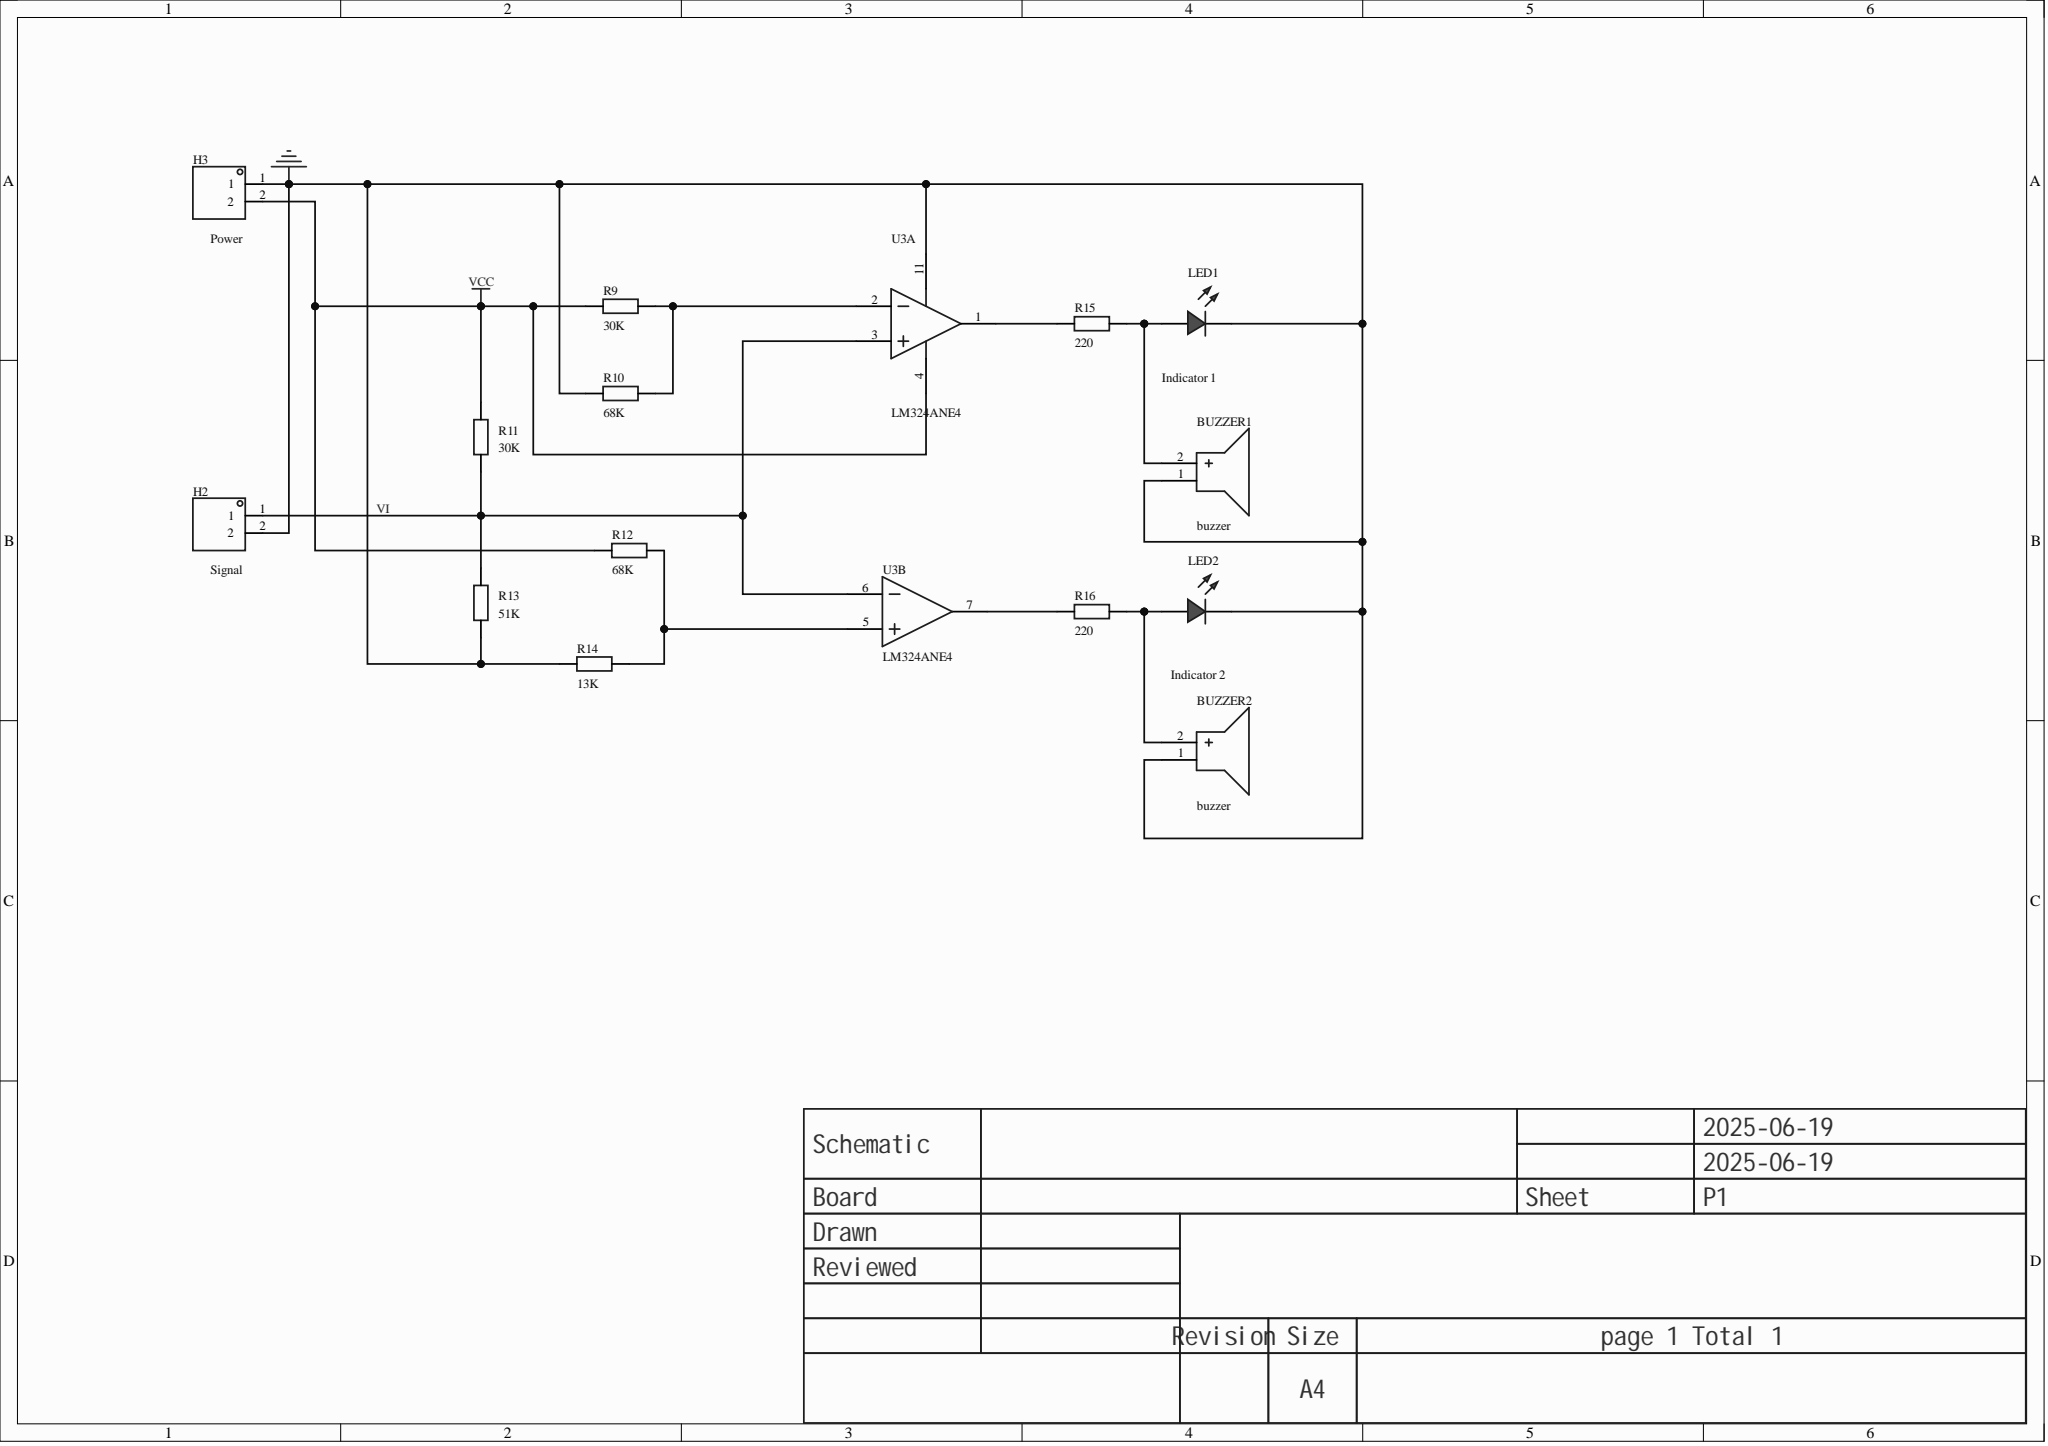Circuit board | Altium Designer | 15 parts | 9 nets
Bill of materials:
Comment,Description,Designator,Footprint,LibRef,Quantity
"buzzer","","BUZZER1, BUZZER2","BUZ-TH_BD12.0-P6.00-D0.9-RD","buzzer","2"
"","","H2, H3","HDR-TH_2P-P2.54-V-M-1","HDR-M_2.54_1x2P","2"
"","","LED1, LED2","LED_TH-3mm","LED_TH-R_3mm","2"
"30K","","R9, R11","Res_1/8W","Res_AXIAL-1/8W","2"
"68K","","R10, R12","Res_1/8W","Res_AXIAL-1/8W","2"
"51K","","R13","Res_1/8W","Res_AXIAL-1/8W","1"
"13K","","R14","Res_1/8W","Res_AXIAL-1/8W","1"
"220","","R15, R16","Res_1/8W","Res_AXIAL-1/8W","2"
"LM324ANE4","","U3","PDIP-14_L19.6-W6.5-P2.54-LS7.9-BL","LM324ANE4","1"
Netlist (Protel format):
[
BUZZER1
BUZ-TH_BD12.0-P6.00-D0.9-RD
buzzer



]
[
BUZZER2
BUZ-TH_BD12.0-P6.00-D0.9-RD
buzzer



]
[
H2
HDR-TH_2P-P2.54-V-M-1




]
[
H3
HDR-TH_2P-P2.54-V-M-1




]
[
LED1
LED_TH-3mm




]
[
LED2
LED_TH-3mm




]
[
R9
Res_1/8W
30K



]
[
R10
Res_1/8W
68K



]
[
R11
Res_1/8W
30K



]
[
R12
Res_1/8W
68K



]
[
R13
Res_1/8W
51K



]
[
R14
Res_1/8W
13K



]
[
R15
Res_1/8W
220



]
[
R16
Res_1/8W
220



]
[
U3
PDIP-14_L19.6-W6.5-P2.54-LS7.9-BL
LM324ANE4



]
(
VI
H2-1
R11-1
R13-2
U3-3
U3-6
)
(
VCC
H3-2
R9-1
R11-2
R12-1
U3-4
)
(
NetR16_1
R16-1
U3-7
)
(
NetR15_1
R15-1
U3-1
)
(
NetR12_2
R12-2
R14-2
U3-5
)
(
NetR9_2
R9-2
R10-2
U3-2
)
(
NetBUZZER2_2
BUZZER2-2
LED2-1
R16-2
)
(
NetBUZZER1_2
BUZZER1-2
LED1-1
R15-2
)
(
GND
BUZZER1-1
BUZZER2-1
H2-2
H3-1
LED1-2
LED2-2
R10-1
R13-1
R14-1
U3-11
)